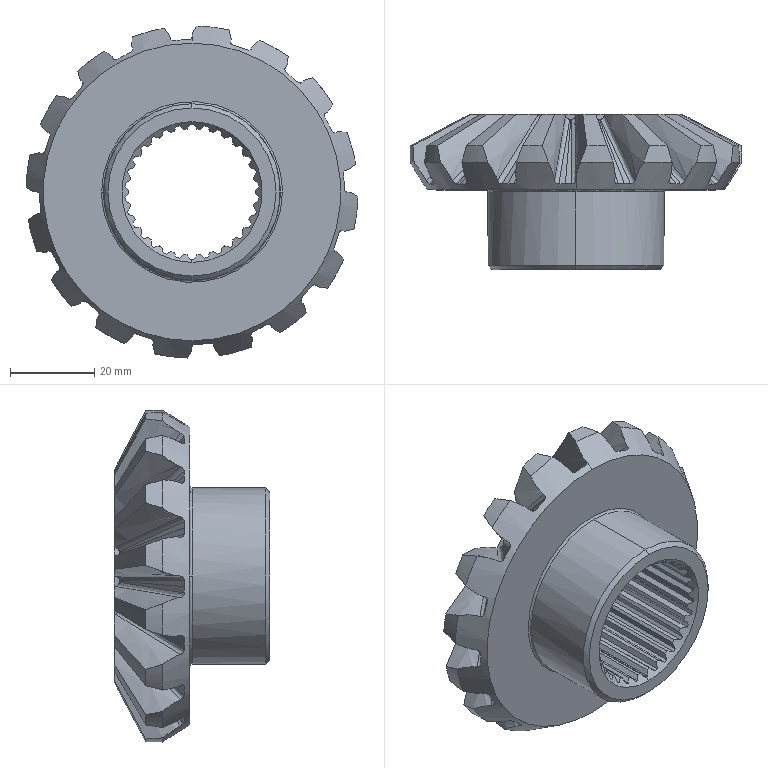Part | SolidWorks | features BaseBody 1 | 1 solid | 281 faces | box 78.97 x 37 x 78.97 mm | volume 57789 mm3 | spline 98 | cylinder 96 | plane 63 | cone 24 | commonest cylinder face diameters 32 x31 30 x30 35.118 x17 79 x16 42 x2